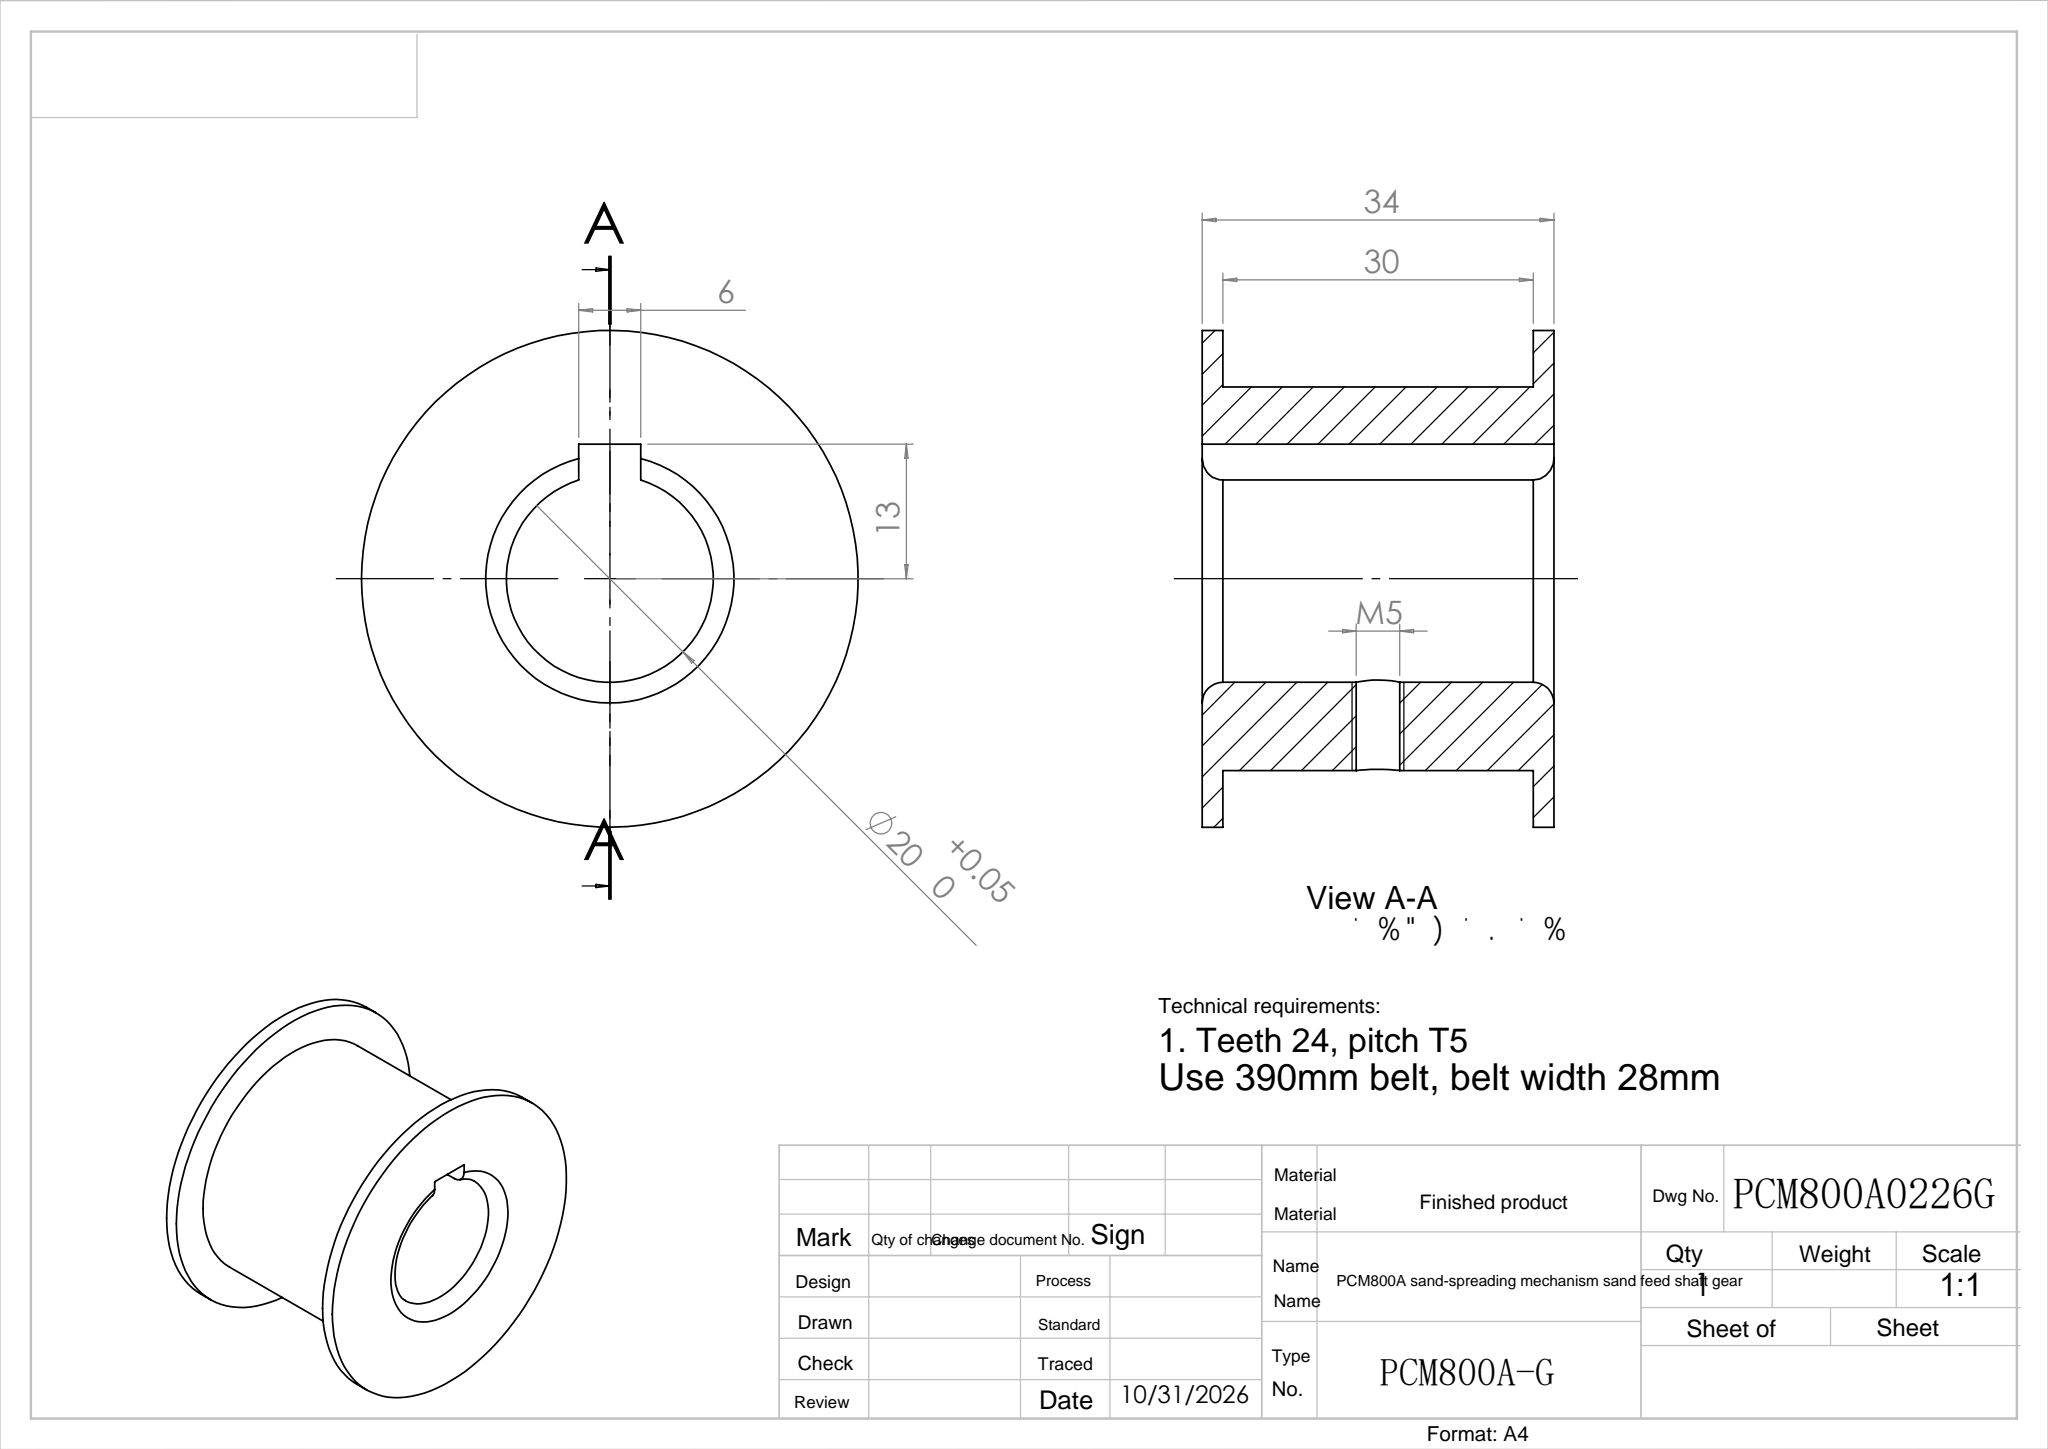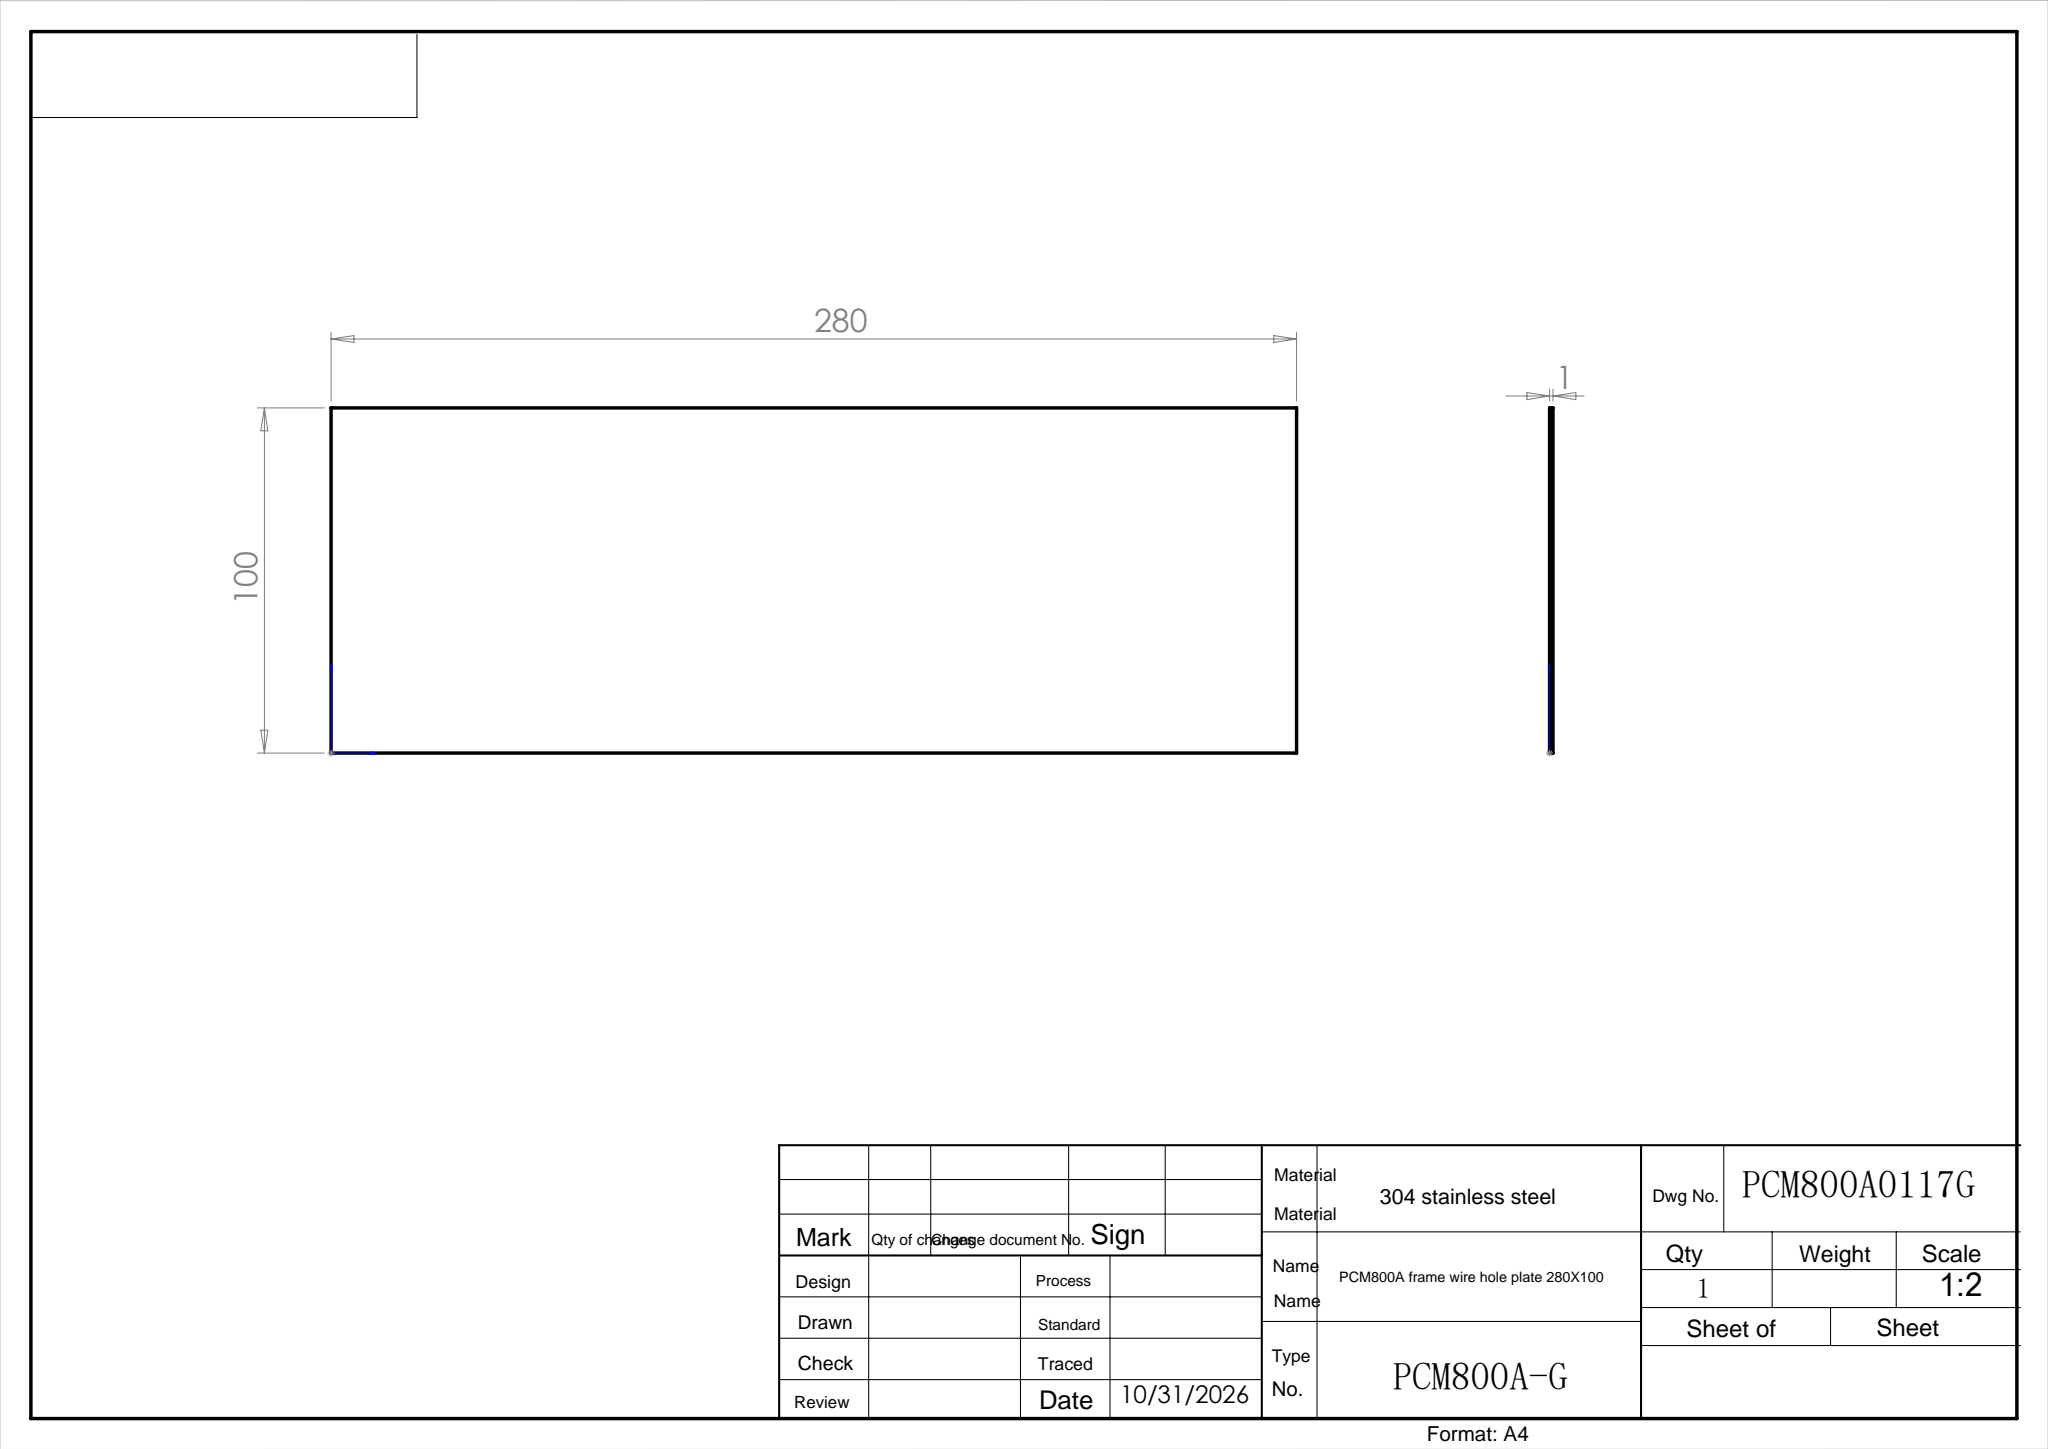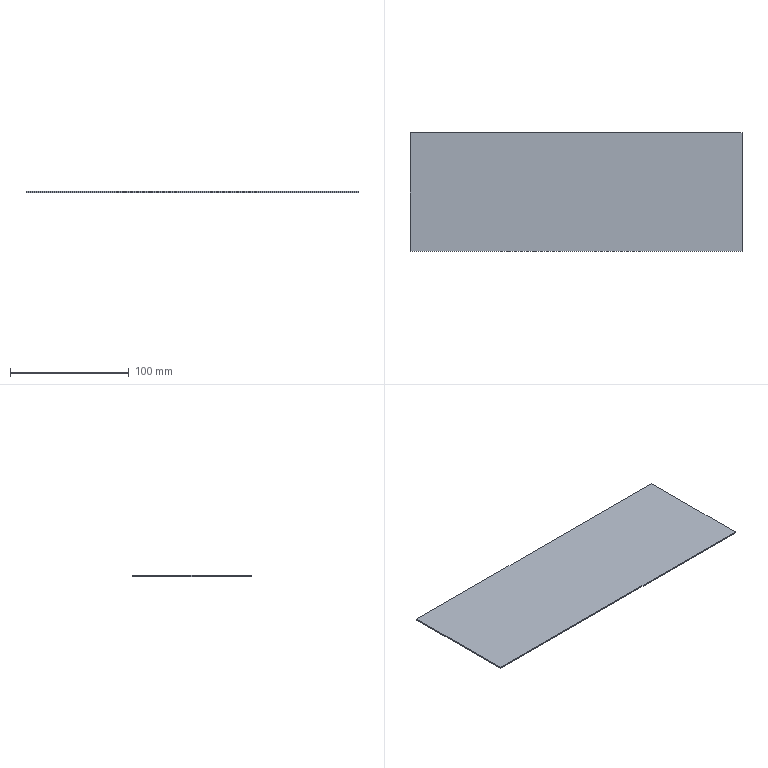Part | SolidWorks | features Extrusion 1 | 1 solid | 6 faces | box 280 x 100 x 1 mm | volume 28000 mm3 | plane 6
STEP:
#1=CARTESIAN_POINT('',(0.,100.,0.));
#2=VERTEX_POINT('',#1);
#3=CARTESIAN_POINT('',(0.,0.,0.));
#4=VERTEX_POINT('',#3);
#5=CARTESIAN_POINT('',(0.,0.,0.));
#6=DIRECTION('',(0.,-1.,0.));
#7=VECTOR('',#6,1000.);
#8=LINE('',#5,#7);
#9=EDGE_CURVE('',#2,#4,#8,.T.);
#10=ORIENTED_EDGE('',*,*,#9,.T.);
#11=CARTESIAN_POINT('',(0.,0.,1.));
#12=VERTEX_POINT('',#11);
#13=CARTESIAN_POINT('',(0.,0.,1.));
#14=DIRECTION('',(0.,0.,-1.));
#15=VECTOR('',#14,1000.);
#16=LINE('',#13,#15);
#17=EDGE_CURVE('',#12,#4,#16,.T.);
#18=ORIENTED_EDGE('',*,*,#17,.F.);
#19=CARTESIAN_POINT('',(0.,100.,1.));
#20=VERTEX_POINT('',#19);
#21=CARTESIAN_POINT('',(0.,0.,1.));
#22=DIRECTION('',(0.,-1.,0.));
#23=VECTOR('',#22,1000.);
#24=LINE('',#21,#23);
#25=EDGE_CURVE('',#20,#12,#24,.T.);
#26=ORIENTED_EDGE('',*,*,#25,.F.);
#27=CARTESIAN_POINT('',(0.,100.,1.));
#28=DIRECTION('',(0.,0.,-1.));
#29=VECTOR('',#28,1000.);
#30=LINE('',#27,#29);
#31=EDGE_CURVE('',#20,#2,#30,.T.);
#32=ORIENTED_EDGE('',*,*,#31,.T.);
#33=EDGE_LOOP('',(#10,#18,#26,#32));
#34=FACE_OUTER_BOUND('',#33,.T.);
#35=CARTESIAN_POINT('',(0.,0.,1.));
#36=DIRECTION('',(1.,0.,0.));
#37=DIRECTION('',(0.,1.,0.));
#38=AXIS2_PLACEMENT_3D('',#35,#36,#37);
#39=PLANE('',#38);
#40=ADVANCED_FACE('',(#34),#39,.F.);
#41=CARTESIAN_POINT('',(280.,0.,0.));
#42=VERTEX_POINT('',#41);
#43=CARTESIAN_POINT('',(0.,0.,0.));
#44=DIRECTION('',(1.,0.,0.));
#45=VECTOR('',#44,1000.);
#46=LINE('',#43,#45);
#47=EDGE_CURVE('',#4,#42,#46,.T.);
#48=ORIENTED_EDGE('',*,*,#47,.T.);
#49=CARTESIAN_POINT('',(280.,0.,1.));
#50=VERTEX_POINT('',#49);
#51=CARTESIAN_POINT('',(280.,0.,1.));
#52=DIRECTION('',(0.,0.,-1.));
#53=VECTOR('',#52,1000.);
#54=LINE('',#51,#53);
#55=EDGE_CURVE('',#50,#42,#54,.T.);
#56=ORIENTED_EDGE('',*,*,#55,.F.);
#57=CARTESIAN_POINT('',(0.,0.,1.));
#58=DIRECTION('',(1.,0.,0.));
#59=VECTOR('',#58,1000.);
#60=LINE('',#57,#59);
#61=EDGE_CURVE('',#12,#50,#60,.T.);
#62=ORIENTED_EDGE('',*,*,#61,.F.);
#63=ORIENTED_EDGE('',*,*,#17,.T.);
#64=EDGE_LOOP('',(#48,#56,#62,#63));
#65=FACE_OUTER_BOUND('',#64,.T.);
#66=CARTESIAN_POINT('',(0.,0.,1.));
#67=DIRECTION('',(0.,1.,0.));
#68=DIRECTION('',(0.,0.,1.));
#69=AXIS2_PLACEMENT_3D('',#66,#67,#68);
#70=PLANE('',#69);
#71=ADVANCED_FACE('',(#65),#70,.F.);
#72=CARTESIAN_POINT('',(280.,100.,0.));
#73=VERTEX_POINT('',#72);
#74=CARTESIAN_POINT('',(280.,0.,0.));
#75=DIRECTION('',(0.,1.,0.));
#76=VECTOR('',#75,1000.);
#77=LINE('',#74,#76);
#78=EDGE_CURVE('',#42,#73,#77,.T.);
#79=ORIENTED_EDGE('',*,*,#78,.T.);
#80=CARTESIAN_POINT('',(280.,100.,1.));
#81=VERTEX_POINT('',#80);
#82=CARTESIAN_POINT('',(280.,100.,1.));
#83=DIRECTION('',(0.,0.,-1.));
#84=VECTOR('',#83,1000.);
#85=LINE('',#82,#84);
#86=EDGE_CURVE('',#81,#73,#85,.T.);
#87=ORIENTED_EDGE('',*,*,#86,.F.);
#88=CARTESIAN_POINT('',(280.,0.,1.));
#89=DIRECTION('',(0.,1.,0.));
#90=VECTOR('',#89,1000.);
#91=LINE('',#88,#90);
#92=EDGE_CURVE('',#50,#81,#91,.T.);
#93=ORIENTED_EDGE('',*,*,#92,.F.);
#94=ORIENTED_EDGE('',*,*,#55,.T.);
#95=EDGE_LOOP('',(#79,#87,#93,#94));
#96=FACE_OUTER_BOUND('',#95,.T.);
#97=CARTESIAN_POINT('',(280.,0.,1.));
#98=DIRECTION('',(-1.,0.,0.));
#99=DIRECTION('',(0.,0.,1.));
#100=AXIS2_PLACEMENT_3D('',#97,#98,#99);
#101=PLANE('',#100);
#102=ADVANCED_FACE('',(#96),#101,.F.);
#103=CARTESIAN_POINT('',(0.,100.,0.));
#104=DIRECTION('',(-1.,0.,0.));
#105=VECTOR('',#104,1000.);
#106=LINE('',#103,#105);
#107=EDGE_CURVE('',#73,#2,#106,.T.);
#108=ORIENTED_EDGE('',*,*,#107,.T.);
#109=ORIENTED_EDGE('',*,*,#31,.F.);
#110=CARTESIAN_POINT('',(0.,100.,1.));
#111=DIRECTION('',(-1.,0.,0.));
#112=VECTOR('',#111,1000.);
#113=LINE('',#110,#112);
#114=EDGE_CURVE('',#81,#20,#113,.T.);
#115=ORIENTED_EDGE('',*,*,#114,.F.);
#116=ORIENTED_EDGE('',*,*,#86,.T.);
#117=EDGE_LOOP('',(#108,#109,#115,#116));
#118=FACE_OUTER_BOUND('',#117,.T.);
#119=CARTESIAN_POINT('',(0.,100.,1.));
#120=DIRECTION('',(0.,-1.,0.));
#121=DIRECTION('',(0.,0.,-1.));
#122=AXIS2_PLACEMENT_3D('',#119,#120,#121);
#123=PLANE('',#122);
#124=ADVANCED_FACE('',(#118),#123,.F.);
#125=ORIENTED_EDGE('',*,*,#25,.T.);
#126=ORIENTED_EDGE('',*,*,#61,.T.);
#127=ORIENTED_EDGE('',*,*,#92,.T.);
#128=ORIENTED_EDGE('',*,*,#114,.T.);
#129=EDGE_LOOP('',(#125,#126,#127,#128));
#130=FACE_OUTER_BOUND('',#129,.T.);
#131=CARTESIAN_POINT('',(0.,100.,1.));
#132=DIRECTION('',(0.,0.,-1.));
#133=DIRECTION('',(-1.,0.,0.));
#134=AXIS2_PLACEMENT_3D('',#131,#132,#133);
#135=PLANE('',#134);
#136=ADVANCED_FACE('',(#130),#135,.F.);
#137=ORIENTED_EDGE('',*,*,#9,.F.);
#138=ORIENTED_EDGE('',*,*,#107,.F.);
#139=ORIENTED_EDGE('',*,*,#78,.F.);
#140=ORIENTED_EDGE('',*,*,#47,.F.);
#141=EDGE_LOOP('',(#137,#138,#139,#140));
#142=FACE_OUTER_BOUND('',#141,.T.);
#143=CARTESIAN_POINT('',(0.,100.,0.));
#144=DIRECTION('',(0.,0.,-1.));
#145=DIRECTION('',(-1.,0.,0.));
#146=AXIS2_PLACEMENT_3D('',#143,#144,#145);
#147=PLANE('',#146);
#148=ADVANCED_FACE('',(#142),#147,.T.);
#149=CLOSED_SHELL('',(#40,#71,#102,#124,#136,#148));
#150=MANIFOLD_SOLID_BREP('',#149);
#151=CARTESIAN_POINT('',(0.,0.,0.));
#152=DIRECTION('',(0.,0.,1.));
#153=DIRECTION('',(1.,0.,0.));
#154=AXIS2_PLACEMENT_3D('',#151,#152,#153);
#155=(LENGTH_UNIT()NAMED_UNIT(*)SI_UNIT(.MILLI.,.METRE.));
#156=UNCERTAINTY_MEASURE_WITH_UNIT(LENGTH_MEASURE(0.00001),#155,'','');
#157=(NAMED_UNIT(*)PLANE_ANGLE_UNIT()SI_UNIT($,.RADIAN.));
#158=(NAMED_UNIT(*)SI_UNIT($,.STERADIAN.)SOLID_ANGLE_UNIT());
#159=(GEOMETRIC_REPRESENTATION_CONTEXT(3)GLOBAL_UNCERTAINTY_ASSIGNED_CONTEXT((#156))GLOBAL_UNIT_ASSIGNED_CONTEXT((#155,#157,#158))REPRESENTATION_CONTEXT('',''));
#160=ADVANCED_BREP_SHAPE_REPRESENTATION('',(#150,#154),#159);